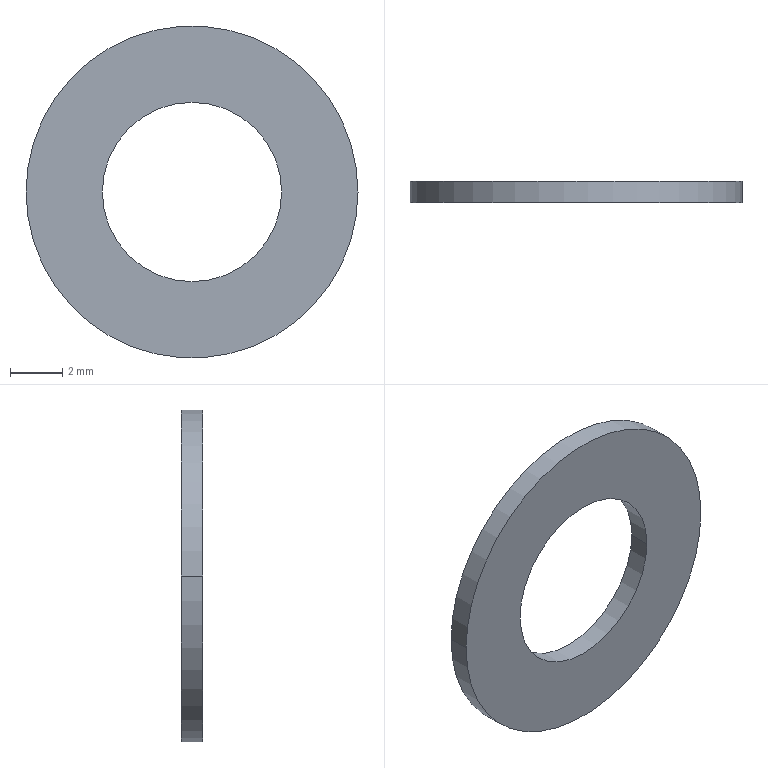Part | NX | features BREP 1 | 1 solid | 6 faces | box 12.7 x 0.8128 x 12.7 mm | volume 72.939 mm3 | cylinder 4 | plane 2 | commonest cylinder face diameters 6.858 x2 12.7 x2
STEP:
#1=CARTESIAN_POINT('',(-6.35,0.,0.));
#2=VERTEX_POINT('',#1);
#3=CARTESIAN_POINT('',(6.35,0.,0.));
#4=VERTEX_POINT('',#3);
#5=CARTESIAN_POINT('',(0.,0.,0.));
#6=DIRECTION('',(0.,1.,0.));
#7=DIRECTION('',(-1.,0.,0.));
#8=AXIS2_PLACEMENT_3D('',#5,#6,#7);
#9=CIRCLE('',#8,6.35);
#10=EDGE_CURVE('',#2,#4,#9,.T.);
#11=ORIENTED_EDGE('',*,*,#10,.F.);
#12=CARTESIAN_POINT('',(0.,0.,0.));
#13=DIRECTION('',(0.,1.,0.));
#14=DIRECTION('',(1.,0.,0.));
#15=AXIS2_PLACEMENT_3D('',#12,#13,#14);
#16=CIRCLE('',#15,6.35);
#17=EDGE_CURVE('',#4,#2,#16,.T.);
#18=ORIENTED_EDGE('',*,*,#17,.F.);
#19=EDGE_LOOP('',(#11,#18));
#20=FACE_BOUND('',#19,.T.);
#21=CARTESIAN_POINT('',(-3.429,0.,0.));
#22=VERTEX_POINT('',#21);
#23=CARTESIAN_POINT('',(3.429,0.,0.));
#24=VERTEX_POINT('',#23);
#25=CARTESIAN_POINT('',(0.,0.,0.));
#26=DIRECTION('',(0.,-1.,0.));
#27=DIRECTION('',(-1.,0.,0.));
#28=AXIS2_PLACEMENT_3D('',#25,#26,#27);
#29=CIRCLE('',#28,3.429);
#30=EDGE_CURVE('',#22,#24,#29,.T.);
#31=ORIENTED_EDGE('',*,*,#30,.F.);
#32=CARTESIAN_POINT('',(0.,0.,0.));
#33=DIRECTION('',(0.,-1.,0.));
#34=DIRECTION('',(1.,0.,0.));
#35=AXIS2_PLACEMENT_3D('',#32,#33,#34);
#36=CIRCLE('',#35,3.429);
#37=EDGE_CURVE('',#24,#22,#36,.T.);
#38=ORIENTED_EDGE('',*,*,#37,.F.);
#39=EDGE_LOOP('',(#31,#38));
#40=FACE_BOUND('',#39,.T.);
#41=CARTESIAN_POINT('',(0.,0.,0.));
#42=DIRECTION('',(0.,1.,0.));
#43=DIRECTION('',(1.,0.,0.));
#44=AXIS2_PLACEMENT_3D('',#41,#42,#43);
#45=PLANE('',#44);
#46=ADVANCED_FACE('',(#20,#40),#45,.F.);
#47=CARTESIAN_POINT('',(-6.35,0.8128,0.));
#48=VERTEX_POINT('',#47);
#49=CARTESIAN_POINT('',(-6.35,0.,0.));
#50=DIRECTION('',(0.,1.,0.));
#51=VECTOR('',#50,1000.);
#52=LINE('',#49,#51);
#53=EDGE_CURVE('',#2,#48,#52,.T.);
#54=ORIENTED_EDGE('',*,*,#53,.T.);
#55=CARTESIAN_POINT('',(6.35,0.8128,0.));
#56=VERTEX_POINT('',#55);
#57=CARTESIAN_POINT('',(0.,0.8128,0.));
#58=DIRECTION('',(0.,1.,0.));
#59=DIRECTION('',(1.,0.,0.));
#60=AXIS2_PLACEMENT_3D('',#57,#58,#59);
#61=CIRCLE('',#60,6.35);
#62=EDGE_CURVE('',#56,#48,#61,.T.);
#63=ORIENTED_EDGE('',*,*,#62,.F.);
#64=CARTESIAN_POINT('',(6.35,0.,0.));
#65=DIRECTION('',(0.,1.,0.));
#66=VECTOR('',#65,1000.);
#67=LINE('',#64,#66);
#68=EDGE_CURVE('',#4,#56,#67,.T.);
#69=ORIENTED_EDGE('',*,*,#68,.F.);
#70=ORIENTED_EDGE('',*,*,#17,.T.);
#71=EDGE_LOOP('',(#54,#63,#69,#70));
#72=FACE_BOUND('',#71,.T.);
#73=CARTESIAN_POINT('',(0.,0.,0.));
#74=DIRECTION('',(0.,1.,0.));
#75=DIRECTION('',(1.,0.,0.));
#76=AXIS2_PLACEMENT_3D('',#73,#74,#75);
#77=CYLINDRICAL_SURFACE('',#76,6.35);
#78=ADVANCED_FACE('',(#72),#77,.T.);
#79=ORIENTED_EDGE('',*,*,#68,.T.);
#80=CARTESIAN_POINT('',(0.,0.8128,0.));
#81=DIRECTION('',(0.,1.,0.));
#82=DIRECTION('',(-1.,0.,0.));
#83=AXIS2_PLACEMENT_3D('',#80,#81,#82);
#84=CIRCLE('',#83,6.35);
#85=EDGE_CURVE('',#48,#56,#84,.T.);
#86=ORIENTED_EDGE('',*,*,#85,.F.);
#87=ORIENTED_EDGE('',*,*,#53,.F.);
#88=ORIENTED_EDGE('',*,*,#10,.T.);
#89=EDGE_LOOP('',(#79,#86,#87,#88));
#90=FACE_BOUND('',#89,.T.);
#91=CARTESIAN_POINT('',(0.,0.,0.));
#92=DIRECTION('',(0.,1.,0.));
#93=DIRECTION('',(1.,0.,0.));
#94=AXIS2_PLACEMENT_3D('',#91,#92,#93);
#95=CYLINDRICAL_SURFACE('',#94,6.35);
#96=ADVANCED_FACE('',(#90),#95,.T.);
#97=ORIENTED_EDGE('',*,*,#85,.T.);
#98=ORIENTED_EDGE('',*,*,#62,.T.);
#99=EDGE_LOOP('',(#97,#98));
#100=FACE_BOUND('',#99,.T.);
#101=CARTESIAN_POINT('',(-3.429,0.8128,0.));
#102=VERTEX_POINT('',#101);
#103=CARTESIAN_POINT('',(3.429,0.8128,0.));
#104=VERTEX_POINT('',#103);
#105=CARTESIAN_POINT('',(0.,0.8128,0.));
#106=DIRECTION('',(0.,-1.,0.));
#107=DIRECTION('',(-1.,0.,0.));
#108=AXIS2_PLACEMENT_3D('',#105,#106,#107);
#109=CIRCLE('',#108,3.429);
#110=EDGE_CURVE('',#102,#104,#109,.T.);
#111=ORIENTED_EDGE('',*,*,#110,.T.);
#112=CARTESIAN_POINT('',(0.,0.8128,0.));
#113=DIRECTION('',(0.,-1.,0.));
#114=DIRECTION('',(1.,0.,0.));
#115=AXIS2_PLACEMENT_3D('',#112,#113,#114);
#116=CIRCLE('',#115,3.429);
#117=EDGE_CURVE('',#104,#102,#116,.T.);
#118=ORIENTED_EDGE('',*,*,#117,.T.);
#119=EDGE_LOOP('',(#111,#118));
#120=FACE_BOUND('',#119,.T.);
#121=CARTESIAN_POINT('',(0.,0.8128,0.));
#122=DIRECTION('',(0.,1.,0.));
#123=DIRECTION('',(1.,0.,0.));
#124=AXIS2_PLACEMENT_3D('',#121,#122,#123);
#125=PLANE('',#124);
#126=ADVANCED_FACE('',(#100,#120),#125,.T.);
#127=CARTESIAN_POINT('',(-3.429,0.,0.));
#128=DIRECTION('',(0.,1.,0.));
#129=VECTOR('',#128,1000.);
#130=LINE('',#127,#129);
#131=EDGE_CURVE('',#22,#102,#130,.T.);
#132=ORIENTED_EDGE('',*,*,#131,.T.);
#133=ORIENTED_EDGE('',*,*,#117,.F.);
#134=CARTESIAN_POINT('',(3.429,0.,0.));
#135=DIRECTION('',(0.,1.,0.));
#136=VECTOR('',#135,1000.);
#137=LINE('',#134,#136);
#138=EDGE_CURVE('',#24,#104,#137,.T.);
#139=ORIENTED_EDGE('',*,*,#138,.F.);
#140=ORIENTED_EDGE('',*,*,#37,.T.);
#141=EDGE_LOOP('',(#132,#133,#139,#140));
#142=FACE_BOUND('',#141,.T.);
#143=CARTESIAN_POINT('',(0.,0.,0.));
#144=DIRECTION('',(0.,1.,0.));
#145=DIRECTION('',(1.,0.,0.));
#146=AXIS2_PLACEMENT_3D('',#143,#144,#145);
#147=CYLINDRICAL_SURFACE('',#146,3.429);
#148=ADVANCED_FACE('',(#142),#147,.F.);
#149=ORIENTED_EDGE('',*,*,#138,.T.);
#150=ORIENTED_EDGE('',*,*,#110,.F.);
#151=ORIENTED_EDGE('',*,*,#131,.F.);
#152=ORIENTED_EDGE('',*,*,#30,.T.);
#153=EDGE_LOOP('',(#149,#150,#151,#152));
#154=FACE_BOUND('',#153,.T.);
#155=CARTESIAN_POINT('',(0.,0.,0.));
#156=DIRECTION('',(0.,1.,0.));
#157=DIRECTION('',(1.,0.,0.));
#158=AXIS2_PLACEMENT_3D('',#155,#156,#157);
#159=CYLINDRICAL_SURFACE('',#158,3.429);
#160=ADVANCED_FACE('',(#154),#159,.F.);
#161=CLOSED_SHELL('',(#46,#78,#96,#126,#148,#160));
#162=MANIFOLD_SOLID_BREP('',#161);
#163=(LENGTH_UNIT()NAMED_UNIT(*)SI_UNIT(.MILLI.,.METRE.));
#164=UNCERTAINTY_MEASURE_WITH_UNIT(LENGTH_MEASURE(0.00001),#163,'','');
#165=(NAMED_UNIT(*)PLANE_ANGLE_UNIT()SI_UNIT($,.RADIAN.));
#166=(NAMED_UNIT(*)SI_UNIT($,.STERADIAN.)SOLID_ANGLE_UNIT());
#167=(GEOMETRIC_REPRESENTATION_CONTEXT(3)GLOBAL_UNCERTAINTY_ASSIGNED_CONTEXT((#164))GLOBAL_UNIT_ASSIGNED_CONTEXT((#163,#165,#166))REPRESENTATION_CONTEXT('',''));
#168=ADVANCED_BREP_SHAPE_REPRESENTATION('',(#162),#167);